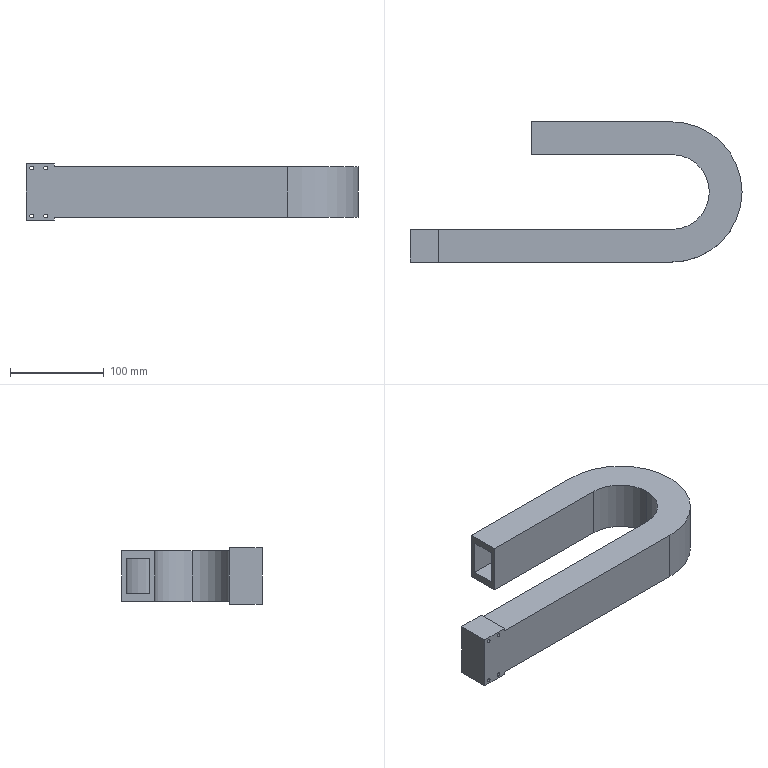Part | STEP file | PN_0019 tank chain, outer 35x54, inner 25x38 | 1 solid | 35 faces | box 355 x 150 x 60 mm | volume 607044 mm3 | plane 19 | cylinder 16 | commonest cylinder face diameters 4 x8 80 x2 90 x2 140 x2 150 x2